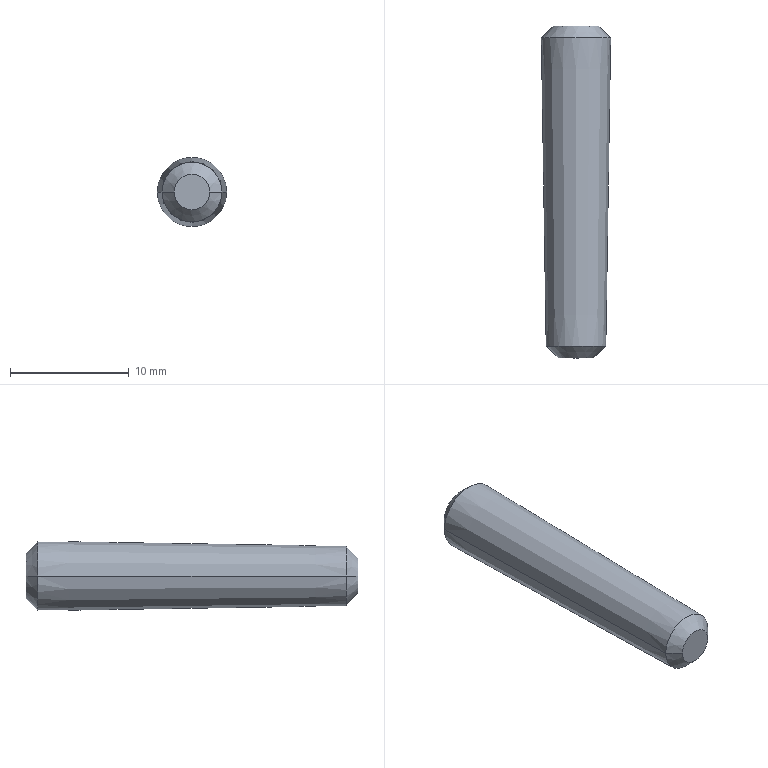Part | NX | features BREP 1 | 1 solid | 8 faces | box 5.848 x 28 x 5.848 mm | volume 637.188 mm3 | cone 6 | plane 2
STEP:
#1=CARTESIAN_POINT('',(1.5,-28.,0.));
#2=VERTEX_POINT('',#1);
#3=CARTESIAN_POINT('',(-1.5,-28.,0.));
#4=VERTEX_POINT('',#3);
#5=CARTESIAN_POINT('',(0.,-28.,0.));
#6=DIRECTION('',(0.,1.,0.));
#7=DIRECTION('',(1.,0.,0.));
#8=AXIS2_PLACEMENT_3D('',#5,#6,#7);
#9=CIRCLE('',#8,1.5);
#10=EDGE_CURVE('',#2,#4,#9,.T.);
#11=ORIENTED_EDGE('',*,*,#10,.F.);
#12=CARTESIAN_POINT('',(0.,-28.,0.));
#13=DIRECTION('',(0.,-1.,0.));
#14=DIRECTION('',(1.,0.,0.));
#15=AXIS2_PLACEMENT_3D('',#12,#13,#14);
#16=CIRCLE('',#15,1.5);
#17=EDGE_CURVE('',#2,#4,#16,.T.);
#18=ORIENTED_EDGE('',*,*,#17,.T.);
#19=EDGE_LOOP('',(#11,#18));
#20=FACE_BOUND('',#19,.T.);
#21=CARTESIAN_POINT('',(0.,-28.,0.));
#22=DIRECTION('',(0.,1.,0.));
#23=DIRECTION('',(-1.,0.,0.));
#24=AXIS2_PLACEMENT_3D('',#21,#22,#23);
#25=PLANE('',#24);
#26=ADVANCED_FACE('',(#20),#25,.F.);
#27=CARTESIAN_POINT('',(-2.516,-27.,0.));
#28=VERTEX_POINT('',#27);
#29=CARTESIAN_POINT('',(-2.516,-27.,0.));
#30=DIRECTION('',(0.7126,-0.7015,0.));
#31=VECTOR('',#30,1000.);
#32=LINE('',#29,#31);
#33=EDGE_CURVE('',#28,#4,#32,.T.);
#34=ORIENTED_EDGE('',*,*,#33,.T.);
#35=ORIENTED_EDGE('',*,*,#17,.F.);
#36=CARTESIAN_POINT('',(2.516,-27.,0.));
#37=VERTEX_POINT('',#36);
#38=CARTESIAN_POINT('',(2.516,-27.,0.));
#39=DIRECTION('',(-0.7126,-0.7015,0.));
#40=VECTOR('',#39,1000.);
#41=LINE('',#38,#40);
#42=EDGE_CURVE('',#37,#2,#41,.T.);
#43=ORIENTED_EDGE('',*,*,#42,.F.);
#44=CARTESIAN_POINT('',(0.,-27.,0.));
#45=DIRECTION('',(0.,-1.,0.));
#46=DIRECTION('',(1.,0.,0.));
#47=AXIS2_PLACEMENT_3D('',#44,#45,#46);
#48=CIRCLE('',#47,2.516);
#49=EDGE_CURVE('',#37,#28,#48,.T.);
#50=ORIENTED_EDGE('',*,*,#49,.T.);
#51=EDGE_LOOP('',(#34,#35,#43,#50));
#52=FACE_BOUND('',#51,.T.);
#53=CARTESIAN_POINT('',(0.,-27.5,0.));
#54=DIRECTION('',(0.,1.,0.));
#55=DIRECTION('',(-1.,0.,0.));
#56=AXIS2_PLACEMENT_3D('',#53,#54,#55);
#57=CONICAL_SURFACE('',#56,2.008,0.7933);
#58=ADVANCED_FACE('',(#52),#57,.T.);
#59=CARTESIAN_POINT('',(2.924,-0.9999,0.));
#60=VERTEX_POINT('',#59);
#61=CARTESIAN_POINT('',(-2.924,-0.9999,0.));
#62=VERTEX_POINT('',#61);
#63=CARTESIAN_POINT('',(0.,-0.9999,0.));
#64=DIRECTION('',(0.,-1.,0.));
#65=DIRECTION('',(1.,0.,0.));
#66=AXIS2_PLACEMENT_3D('',#63,#64,#65);
#67=CIRCLE('',#66,2.924);
#68=EDGE_CURVE('',#60,#62,#67,.T.);
#69=ORIENTED_EDGE('',*,*,#68,.T.);
#70=CARTESIAN_POINT('',(-2.516,-27.,0.));
#71=DIRECTION('',(-0.01571,0.9999,0.));
#72=VECTOR('',#71,1000.);
#73=LINE('',#70,#72);
#74=EDGE_CURVE('',#62,#28,#73,.F.);
#75=ORIENTED_EDGE('',*,*,#74,.T.);
#76=ORIENTED_EDGE('',*,*,#49,.F.);
#77=CARTESIAN_POINT('',(2.516,-27.,0.));
#78=DIRECTION('',(0.01571,0.9999,0.));
#79=VECTOR('',#78,1000.);
#80=LINE('',#77,#79);
#81=EDGE_CURVE('',#60,#37,#80,.F.);
#82=ORIENTED_EDGE('',*,*,#81,.F.);
#83=EDGE_LOOP('',(#69,#75,#76,#82));
#84=FACE_BOUND('',#83,.T.);
#85=CARTESIAN_POINT('',(0.,-14.,0.));
#86=DIRECTION('',(0.,1.,0.));
#87=DIRECTION('',(-1.,0.,0.));
#88=AXIS2_PLACEMENT_3D('',#85,#86,#87);
#89=CONICAL_SURFACE('',#88,2.72,0.01571);
#90=ADVANCED_FACE('',(#84),#89,.T.);
#91=CARTESIAN_POINT('',(0.,-27.,0.));
#92=DIRECTION('',(0.,1.,0.));
#93=DIRECTION('',(1.,0.,0.));
#94=AXIS2_PLACEMENT_3D('',#91,#92,#93);
#95=CIRCLE('',#94,2.516);
#96=EDGE_CURVE('',#37,#28,#95,.T.);
#97=ORIENTED_EDGE('',*,*,#96,.T.);
#98=ORIENTED_EDGE('',*,*,#74,.F.);
#99=CARTESIAN_POINT('',(0.,-0.9999,0.));
#100=DIRECTION('',(0.,1.,0.));
#101=DIRECTION('',(1.,0.,0.));
#102=AXIS2_PLACEMENT_3D('',#99,#100,#101);
#103=CIRCLE('',#102,2.924);
#104=EDGE_CURVE('',#60,#62,#103,.T.);
#105=ORIENTED_EDGE('',*,*,#104,.F.);
#106=ORIENTED_EDGE('',*,*,#81,.T.);
#107=EDGE_LOOP('',(#97,#98,#105,#106));
#108=FACE_BOUND('',#107,.T.);
#109=CARTESIAN_POINT('',(0.,-14.,0.));
#110=DIRECTION('',(0.,1.,0.));
#111=DIRECTION('',(-1.,0.,0.));
#112=AXIS2_PLACEMENT_3D('',#109,#110,#111);
#113=CONICAL_SURFACE('',#112,2.72,0.01571);
#114=ADVANCED_FACE('',(#108),#113,.T.);
#115=CARTESIAN_POINT('',(1.94,0.,0.));
#116=VERTEX_POINT('',#115);
#117=CARTESIAN_POINT('',(1.94,0.,0.));
#118=DIRECTION('',(0.7015,-0.7126,0.));
#119=VECTOR('',#118,1000.);
#120=LINE('',#117,#119);
#121=EDGE_CURVE('',#60,#116,#120,.F.);
#122=ORIENTED_EDGE('',*,*,#121,.F.);
#123=ORIENTED_EDGE('',*,*,#104,.T.);
#124=CARTESIAN_POINT('',(-1.94,0.,0.));
#125=VERTEX_POINT('',#124);
#126=CARTESIAN_POINT('',(-1.94,0.,0.));
#127=DIRECTION('',(-0.7015,-0.7126,0.));
#128=VECTOR('',#127,1000.);
#129=LINE('',#126,#128);
#130=EDGE_CURVE('',#62,#125,#129,.F.);
#131=ORIENTED_EDGE('',*,*,#130,.T.);
#132=CARTESIAN_POINT('',(0.,0.,0.));
#133=DIRECTION('',(0.,1.,0.));
#134=DIRECTION('',(1.,0.,0.));
#135=AXIS2_PLACEMENT_3D('',#132,#133,#134);
#136=CIRCLE('',#135,1.94);
#137=EDGE_CURVE('',#116,#125,#136,.T.);
#138=ORIENTED_EDGE('',*,*,#137,.F.);
#139=EDGE_LOOP('',(#122,#123,#131,#138));
#140=FACE_BOUND('',#139,.T.);
#141=CARTESIAN_POINT('',(0.,-0.4999,0.));
#142=DIRECTION('',(0.,-1.,0.));
#143=DIRECTION('',(1.,0.,0.));
#144=AXIS2_PLACEMENT_3D('',#141,#142,#143);
#145=CONICAL_SURFACE('',#144,2.432,0.7775);
#146=ADVANCED_FACE('',(#140),#145,.T.);
#147=ORIENTED_EDGE('',*,*,#137,.T.);
#148=CARTESIAN_POINT('',(0.,0.,0.));
#149=DIRECTION('',(0.,-1.,0.));
#150=DIRECTION('',(1.,0.,0.));
#151=AXIS2_PLACEMENT_3D('',#148,#149,#150);
#152=CIRCLE('',#151,1.94);
#153=EDGE_CURVE('',#116,#125,#152,.T.);
#154=ORIENTED_EDGE('',*,*,#153,.F.);
#155=EDGE_LOOP('',(#147,#154));
#156=FACE_BOUND('',#155,.T.);
#157=CARTESIAN_POINT('',(0.,0.,0.));
#158=DIRECTION('',(0.,1.,0.));
#159=DIRECTION('',(-1.,0.,0.));
#160=AXIS2_PLACEMENT_3D('',#157,#158,#159);
#161=PLANE('',#160);
#162=ADVANCED_FACE('',(#156),#161,.T.);
#163=ORIENTED_EDGE('',*,*,#130,.F.);
#164=ORIENTED_EDGE('',*,*,#68,.F.);
#165=ORIENTED_EDGE('',*,*,#121,.T.);
#166=ORIENTED_EDGE('',*,*,#153,.T.);
#167=EDGE_LOOP('',(#163,#164,#165,#166));
#168=FACE_BOUND('',#167,.T.);
#169=CARTESIAN_POINT('',(0.,-0.4999,0.));
#170=DIRECTION('',(0.,-1.,0.));
#171=DIRECTION('',(1.,0.,0.));
#172=AXIS2_PLACEMENT_3D('',#169,#170,#171);
#173=CONICAL_SURFACE('',#172,2.432,0.7775);
#174=ADVANCED_FACE('',(#168),#173,.T.);
#175=ORIENTED_EDGE('',*,*,#42,.T.);
#176=ORIENTED_EDGE('',*,*,#10,.T.);
#177=ORIENTED_EDGE('',*,*,#33,.F.);
#178=ORIENTED_EDGE('',*,*,#96,.F.);
#179=EDGE_LOOP('',(#175,#176,#177,#178));
#180=FACE_BOUND('',#179,.T.);
#181=CARTESIAN_POINT('',(0.,-27.5,0.));
#182=DIRECTION('',(0.,1.,0.));
#183=DIRECTION('',(-1.,0.,0.));
#184=AXIS2_PLACEMENT_3D('',#181,#182,#183);
#185=CONICAL_SURFACE('',#184,2.008,0.7933);
#186=ADVANCED_FACE('',(#180),#185,.T.);
#187=CLOSED_SHELL('',(#26,#58,#90,#114,#146,#162,#174,#186));
#188=MANIFOLD_SOLID_BREP('',#187);
#189=(LENGTH_UNIT()NAMED_UNIT(*)SI_UNIT(.MILLI.,.METRE.));
#190=UNCERTAINTY_MEASURE_WITH_UNIT(LENGTH_MEASURE(0.00001),#189,'','');
#191=(NAMED_UNIT(*)PLANE_ANGLE_UNIT()SI_UNIT($,.RADIAN.));
#192=(NAMED_UNIT(*)SI_UNIT($,.STERADIAN.)SOLID_ANGLE_UNIT());
#193=(GEOMETRIC_REPRESENTATION_CONTEXT(3)GLOBAL_UNCERTAINTY_ASSIGNED_CONTEXT((#190))GLOBAL_UNIT_ASSIGNED_CONTEXT((#189,#191,#192))REPRESENTATION_CONTEXT('',''));
#194=ADVANCED_BREP_SHAPE_REPRESENTATION('',(#188),#193);